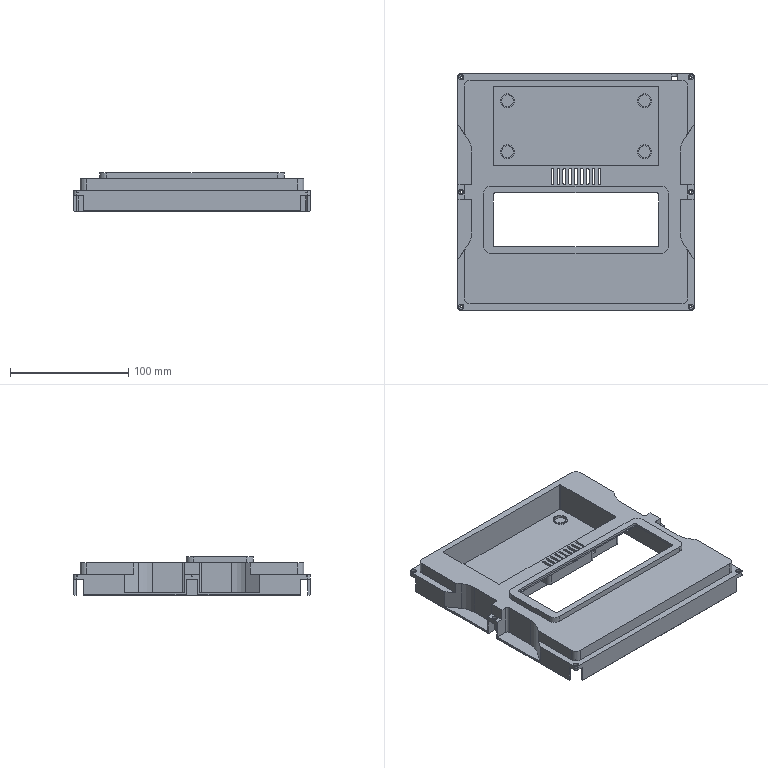Part | SolidWorks | features ICE 30, Fillet 3, Chamfer 1, Extrusion 1, LPattern 1, Shell 1 | 1 solid | 368 faces | box 199.7 x 199.7 x 32.5 mm | volume 138569 mm3 | plane 253 | cylinder 115 | commonest cylinder face diameters 2 x28 4 x14 2.2 x12 4.5 x12 12 x12 10.2 x8